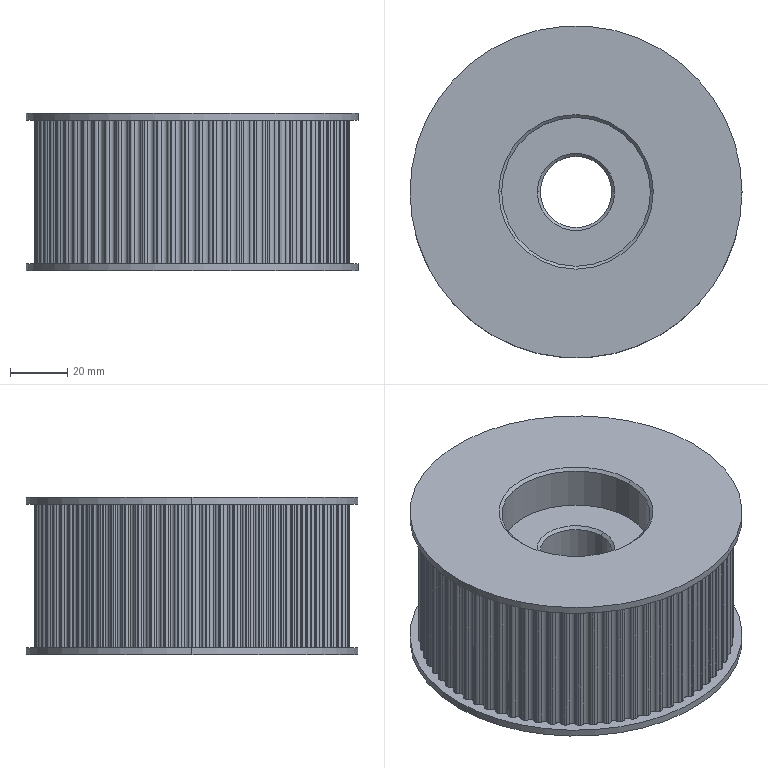Part | 1 solid | 349 faces | box 116 x 116 x 55 mm | volume 440672 mm3 | cylinder 335 | cone 8 | plane 6 | commonest cylinder face diameters 2.5 x254 110 x71 52 x4 116 x4 25 x2